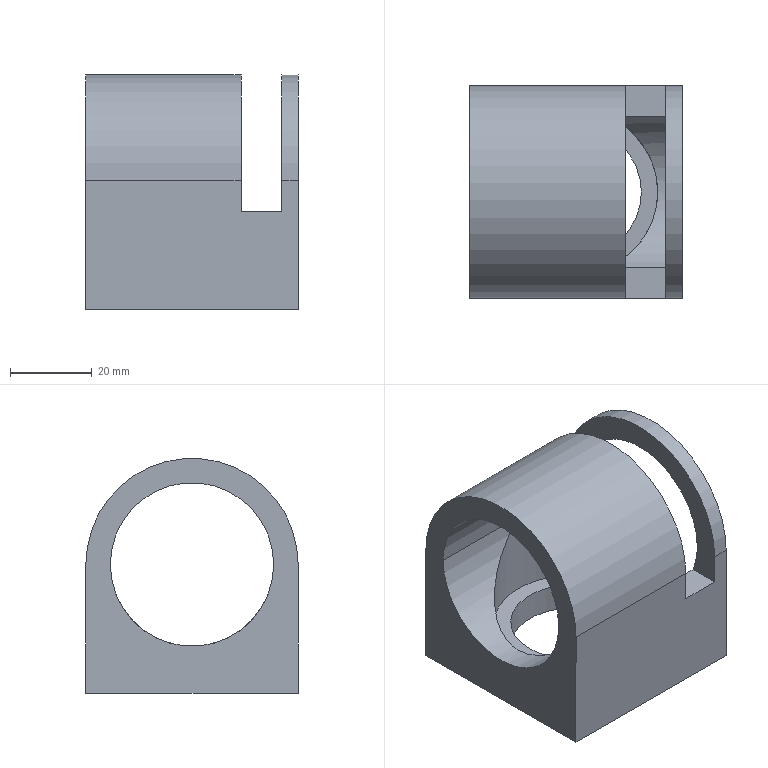Part | SolidWorks | features ICE 8, Extrusion 1 | 1 solid | 35 faces | box 52 x 52 x 57.532 mm | volume 52074 mm3 | cylinder 20 | plane 15 | commonest cylinder face diameters 4 x8 40 x6 32 x2 50 x2 52 x2
STEP:
#1=CARTESIAN_POINT('',(-20.,0.,10.));
#2=VERTEX_POINT('',#1);
#3=CARTESIAN_POINT('',(20.,0.,10.));
#4=VERTEX_POINT('',#3);
#5=CARTESIAN_POINT('',(0.,0.,10.));
#6=DIRECTION('',(0.,0.,1.));
#7=DIRECTION('',(1.,0.,0.));
#8=AXIS2_PLACEMENT_3D('',#5,#6,#7);
#9=CIRCLE('',#8,20.);
#10=EDGE_CURVE('',#2,#4,#9,.T.);
#11=ORIENTED_EDGE('',*,*,#10,.F.);
#12=CARTESIAN_POINT('',(-20.,0.,11.532));
#13=VERTEX_POINT('',#12);
#14=CARTESIAN_POINT('',(-20.,0.,10.));
#15=DIRECTION('',(0.,0.,1.));
#16=VECTOR('',#15,1000.);
#17=LINE('',#14,#16);
#18=EDGE_CURVE('',#2,#13,#17,.T.);
#19=ORIENTED_EDGE('',*,*,#18,.T.);
#20=CARTESIAN_POINT('',(0.,-20.,31.532));
#21=VERTEX_POINT('',#20);
#22=CARTESIAN_POINT('',(-20.,0.,11.532));
#23=CARTESIAN_POINT('',(-20.,-11.716,11.532));
#24=CARTESIAN_POINT('',(-11.716,-20.,19.816));
#25=CARTESIAN_POINT('',(0.,-20.,31.532));
#26=(BOUNDED_CURVE()B_SPLINE_CURVE(3,(#22,#23,#24,#25),.UNSPECIFIED.,.F.,.F.)B_SPLINE_CURVE_WITH_KNOTS((4,4),(3.142,4.712),.UNSPECIFIED.)CURVE()GEOMETRIC_REPRESENTATION_ITEM()RATIONAL_B_SPLINE_CURVE((1.,0.8047,0.8047,1.))REPRESENTATION_ITEM(''));
#27=EDGE_CURVE('',#13,#21,#26,.T.);
#28=ORIENTED_EDGE('',*,*,#27,.T.);
#29=CARTESIAN_POINT('',(20.,0.,11.532));
#30=VERTEX_POINT('',#29);
#31=CARTESIAN_POINT('',(0.,-20.,31.532));
#32=CARTESIAN_POINT('',(11.716,-20.,19.816));
#33=CARTESIAN_POINT('',(20.,-11.716,11.532));
#34=CARTESIAN_POINT('',(20.,0.,11.532));
#35=(BOUNDED_CURVE()B_SPLINE_CURVE(3,(#31,#32,#33,#34),.UNSPECIFIED.,.F.,.F.)B_SPLINE_CURVE_WITH_KNOTS((4,4),(1.571,3.142),.UNSPECIFIED.)CURVE()GEOMETRIC_REPRESENTATION_ITEM()RATIONAL_B_SPLINE_CURVE((1.,0.8047,0.8047,1.))REPRESENTATION_ITEM(''));
#36=EDGE_CURVE('',#21,#30,#35,.T.);
#37=ORIENTED_EDGE('',*,*,#36,.T.);
#38=CARTESIAN_POINT('',(20.,0.,10.));
#39=DIRECTION('',(0.,0.,1.));
#40=VECTOR('',#39,1000.);
#41=LINE('',#38,#40);
#42=EDGE_CURVE('',#4,#30,#41,.T.);
#43=ORIENTED_EDGE('',*,*,#42,.F.);
#44=EDGE_LOOP('',(#11,#19,#28,#37,#43));
#45=FACE_OUTER_BOUND('',#44,.T.);
#46=CARTESIAN_POINT('',(0.,0.,10.));
#47=DIRECTION('',(0.,0.,1.));
#48=DIRECTION('',(1.,0.,0.));
#49=AXIS2_PLACEMENT_3D('',#46,#47,#48);
#50=CYLINDRICAL_SURFACE('',#49,20.);
#51=ADVANCED_FACE('',(#45),#50,.F.);
#52=CARTESIAN_POINT('',(16.,0.,10.));
#53=VERTEX_POINT('',#52);
#54=CARTESIAN_POINT('',(-16.,0.,10.));
#55=VERTEX_POINT('',#54);
#56=CARTESIAN_POINT('',(0.,0.,10.));
#57=DIRECTION('',(0.,0.,-1.));
#58=DIRECTION('',(-1.,0.,0.));
#59=AXIS2_PLACEMENT_3D('',#56,#57,#58);
#60=CIRCLE('',#59,16.);
#61=EDGE_CURVE('',#53,#55,#60,.T.);
#62=ORIENTED_EDGE('',*,*,#61,.F.);
#63=CARTESIAN_POINT('',(16.,0.,3.));
#64=VERTEX_POINT('',#63);
#65=CARTESIAN_POINT('',(16.,0.,10.));
#66=DIRECTION('',(0.,0.,-1.));
#67=VECTOR('',#66,1000.);
#68=LINE('',#65,#67);
#69=EDGE_CURVE('',#53,#64,#68,.T.);
#70=ORIENTED_EDGE('',*,*,#69,.T.);
#71=CARTESIAN_POINT('',(-16.,0.,3.));
#72=VERTEX_POINT('',#71);
#73=CARTESIAN_POINT('',(0.,0.,3.));
#74=DIRECTION('',(0.,0.,-1.));
#75=DIRECTION('',(-1.,0.,0.));
#76=AXIS2_PLACEMENT_3D('',#73,#74,#75);
#77=CIRCLE('',#76,16.);
#78=EDGE_CURVE('',#64,#72,#77,.T.);
#79=ORIENTED_EDGE('',*,*,#78,.T.);
#80=CARTESIAN_POINT('',(-16.,0.,10.));
#81=DIRECTION('',(0.,0.,-1.));
#82=VECTOR('',#81,1000.);
#83=LINE('',#80,#82);
#84=EDGE_CURVE('',#55,#72,#83,.T.);
#85=ORIENTED_EDGE('',*,*,#84,.F.);
#86=EDGE_LOOP('',(#62,#70,#79,#85));
#87=FACE_OUTER_BOUND('',#86,.T.);
#88=CARTESIAN_POINT('',(0.,0.,10.));
#89=DIRECTION('',(0.,0.,-1.));
#90=DIRECTION('',(-1.,0.,0.));
#91=AXIS2_PLACEMENT_3D('',#88,#89,#90);
#92=CYLINDRICAL_SURFACE('',#91,16.);
#93=ADVANCED_FACE('',(#87),#92,.F.);
#94=CARTESIAN_POINT('',(25.,0.,3.));
#95=VERTEX_POINT('',#94);
#96=CARTESIAN_POINT('',(-25.,0.,3.));
#97=VERTEX_POINT('',#96);
#98=CARTESIAN_POINT('',(0.,0.,3.));
#99=DIRECTION('',(0.,0.,-1.));
#100=DIRECTION('',(-1.,0.,0.));
#101=AXIS2_PLACEMENT_3D('',#98,#99,#100);
#102=CIRCLE('',#101,25.);
#103=EDGE_CURVE('',#95,#97,#102,.T.);
#104=ORIENTED_EDGE('',*,*,#103,.F.);
#105=CARTESIAN_POINT('',(25.,0.,0.));
#106=VERTEX_POINT('',#105);
#107=CARTESIAN_POINT('',(25.,0.,3.));
#108=DIRECTION('',(0.,0.,-1.));
#109=VECTOR('',#108,1000.);
#110=LINE('',#107,#109);
#111=EDGE_CURVE('',#95,#106,#110,.T.);
#112=ORIENTED_EDGE('',*,*,#111,.T.);
#113=CARTESIAN_POINT('',(-25.,0.,0.));
#114=VERTEX_POINT('',#113);
#115=CARTESIAN_POINT('',(0.,0.,0.));
#116=DIRECTION('',(0.,0.,-1.));
#117=DIRECTION('',(-1.,0.,0.));
#118=AXIS2_PLACEMENT_3D('',#115,#116,#117);
#119=CIRCLE('',#118,25.);
#120=EDGE_CURVE('',#106,#114,#119,.T.);
#121=ORIENTED_EDGE('',*,*,#120,.T.);
#122=CARTESIAN_POINT('',(-25.,0.,3.));
#123=DIRECTION('',(0.,0.,-1.));
#124=VECTOR('',#123,1000.);
#125=LINE('',#122,#124);
#126=EDGE_CURVE('',#97,#114,#125,.T.);
#127=ORIENTED_EDGE('',*,*,#126,.F.);
#128=EDGE_LOOP('',(#104,#112,#121,#127));
#129=FACE_OUTER_BOUND('',#128,.T.);
#130=CARTESIAN_POINT('',(0.,0.,3.));
#131=DIRECTION('',(0.,0.,-1.));
#132=DIRECTION('',(-1.,0.,0.));
#133=AXIS2_PLACEMENT_3D('',#130,#131,#132);
#134=CYLINDRICAL_SURFACE('',#133,25.);
#135=ADVANCED_FACE('',(#129),#134,.F.);
#136=CARTESIAN_POINT('',(23.,-21.,10.));
#137=VERTEX_POINT('',#136);
#138=CARTESIAN_POINT('',(19.,-21.,10.));
#139=VERTEX_POINT('',#138);
#140=CARTESIAN_POINT('',(21.,-21.,10.));
#141=DIRECTION('',(0.,0.,-1.));
#142=DIRECTION('',(1.,0.,0.));
#143=AXIS2_PLACEMENT_3D('',#140,#141,#142);
#144=CIRCLE('',#143,2.);
#145=EDGE_CURVE('',#137,#139,#144,.T.);
#146=ORIENTED_EDGE('',*,*,#145,.F.);
#147=CARTESIAN_POINT('',(23.,-21.,0.));
#148=VERTEX_POINT('',#147);
#149=CARTESIAN_POINT('',(23.,-21.,10.));
#150=DIRECTION('',(0.,0.,-1.));
#151=VECTOR('',#150,1000.);
#152=LINE('',#149,#151);
#153=EDGE_CURVE('',#137,#148,#152,.T.);
#154=ORIENTED_EDGE('',*,*,#153,.T.);
#155=CARTESIAN_POINT('',(19.,-21.,0.));
#156=VERTEX_POINT('',#155);
#157=CARTESIAN_POINT('',(21.,-21.,0.));
#158=DIRECTION('',(0.,0.,-1.));
#159=DIRECTION('',(1.,0.,0.));
#160=AXIS2_PLACEMENT_3D('',#157,#158,#159);
#161=CIRCLE('',#160,2.);
#162=EDGE_CURVE('',#148,#156,#161,.T.);
#163=ORIENTED_EDGE('',*,*,#162,.T.);
#164=CARTESIAN_POINT('',(19.,-21.,10.));
#165=DIRECTION('',(0.,0.,-1.));
#166=VECTOR('',#165,1000.);
#167=LINE('',#164,#166);
#168=EDGE_CURVE('',#139,#156,#167,.T.);
#169=ORIENTED_EDGE('',*,*,#168,.F.);
#170=EDGE_LOOP('',(#146,#154,#163,#169));
#171=FACE_OUTER_BOUND('',#170,.T.);
#172=CARTESIAN_POINT('',(21.,-21.,10.));
#173=DIRECTION('',(0.,0.,-1.));
#174=DIRECTION('',(-1.,0.,0.));
#175=AXIS2_PLACEMENT_3D('',#172,#173,#174);
#176=CYLINDRICAL_SURFACE('',#175,2.);
#177=ADVANCED_FACE('',(#171),#176,.F.);
#178=CARTESIAN_POINT('',(-19.,-21.,10.));
#179=VERTEX_POINT('',#178);
#180=CARTESIAN_POINT('',(-23.,-21.,10.));
#181=VERTEX_POINT('',#180);
#182=CARTESIAN_POINT('',(-21.,-21.,10.));
#183=DIRECTION('',(0.,0.,-1.));
#184=DIRECTION('',(-1.,0.,0.));
#185=AXIS2_PLACEMENT_3D('',#182,#183,#184);
#186=CIRCLE('',#185,2.);
#187=EDGE_CURVE('',#179,#181,#186,.T.);
#188=ORIENTED_EDGE('',*,*,#187,.F.);
#189=CARTESIAN_POINT('',(-19.,-21.,0.));
#190=VERTEX_POINT('',#189);
#191=CARTESIAN_POINT('',(-19.,-21.,10.));
#192=DIRECTION('',(0.,0.,-1.));
#193=VECTOR('',#192,1000.);
#194=LINE('',#191,#193);
#195=EDGE_CURVE('',#179,#190,#194,.T.);
#196=ORIENTED_EDGE('',*,*,#195,.T.);
#197=CARTESIAN_POINT('',(-23.,-21.,0.));
#198=VERTEX_POINT('',#197);
#199=CARTESIAN_POINT('',(-21.,-21.,0.));
#200=DIRECTION('',(0.,0.,-1.));
#201=DIRECTION('',(-1.,0.,0.));
#202=AXIS2_PLACEMENT_3D('',#199,#200,#201);
#203=CIRCLE('',#202,2.);
#204=EDGE_CURVE('',#190,#198,#203,.T.);
#205=ORIENTED_EDGE('',*,*,#204,.T.);
#206=CARTESIAN_POINT('',(-23.,-21.,10.));
#207=DIRECTION('',(0.,0.,-1.));
#208=VECTOR('',#207,1000.);
#209=LINE('',#206,#208);
#210=EDGE_CURVE('',#181,#198,#209,.T.);
#211=ORIENTED_EDGE('',*,*,#210,.F.);
#212=EDGE_LOOP('',(#188,#196,#205,#211));
#213=FACE_OUTER_BOUND('',#212,.T.);
#214=CARTESIAN_POINT('',(-21.,-21.,10.));
#215=DIRECTION('',(0.,0.,-1.));
#216=DIRECTION('',(-1.,0.,0.));
#217=AXIS2_PLACEMENT_3D('',#214,#215,#216);
#218=CYLINDRICAL_SURFACE('',#217,2.);
#219=ADVANCED_FACE('',(#213),#218,.F.);
#220=CARTESIAN_POINT('',(-19.,21.,10.));
#221=VERTEX_POINT('',#220);
#222=CARTESIAN_POINT('',(-23.,21.,10.));
#223=VERTEX_POINT('',#222);
#224=CARTESIAN_POINT('',(-21.,21.,10.));
#225=DIRECTION('',(0.,0.,-1.));
#226=DIRECTION('',(1.,0.,0.));
#227=AXIS2_PLACEMENT_3D('',#224,#225,#226);
#228=CIRCLE('',#227,2.);
#229=EDGE_CURVE('',#221,#223,#228,.T.);
#230=ORIENTED_EDGE('',*,*,#229,.F.);
#231=CARTESIAN_POINT('',(-19.,21.,0.));
#232=VERTEX_POINT('',#231);
#233=CARTESIAN_POINT('',(-19.,21.,10.));
#234=DIRECTION('',(0.,0.,-1.));
#235=VECTOR('',#234,1000.);
#236=LINE('',#233,#235);
#237=EDGE_CURVE('',#221,#232,#236,.T.);
#238=ORIENTED_EDGE('',*,*,#237,.T.);
#239=CARTESIAN_POINT('',(-23.,21.,0.));
#240=VERTEX_POINT('',#239);
#241=CARTESIAN_POINT('',(-21.,21.,0.));
#242=DIRECTION('',(0.,0.,-1.));
#243=DIRECTION('',(1.,0.,0.));
#244=AXIS2_PLACEMENT_3D('',#241,#242,#243);
#245=CIRCLE('',#244,2.);
#246=EDGE_CURVE('',#232,#240,#245,.T.);
#247=ORIENTED_EDGE('',*,*,#246,.T.);
#248=CARTESIAN_POINT('',(-23.,21.,10.));
#249=DIRECTION('',(0.,0.,-1.));
#250=VECTOR('',#249,1000.);
#251=LINE('',#248,#250);
#252=EDGE_CURVE('',#223,#240,#251,.T.);
#253=ORIENTED_EDGE('',*,*,#252,.F.);
#254=EDGE_LOOP('',(#230,#238,#247,#253));
#255=FACE_OUTER_BOUND('',#254,.T.);
#256=CARTESIAN_POINT('',(-21.,21.,10.));
#257=DIRECTION('',(0.,0.,-1.));
#258=DIRECTION('',(-1.,0.,0.));
#259=AXIS2_PLACEMENT_3D('',#256,#257,#258);
#260=CYLINDRICAL_SURFACE('',#259,2.);
#261=ADVANCED_FACE('',(#255),#260,.F.);
#262=CARTESIAN_POINT('',(23.,21.,10.));
#263=VERTEX_POINT('',#262);
#264=CARTESIAN_POINT('',(19.,21.,10.));
#265=VERTEX_POINT('',#264);
#266=CARTESIAN_POINT('',(21.,21.,10.));
#267=DIRECTION('',(0.,0.,-1.));
#268=DIRECTION('',(-1.,0.,0.));
#269=AXIS2_PLACEMENT_3D('',#266,#267,#268);
#270=CIRCLE('',#269,2.);
#271=EDGE_CURVE('',#263,#265,#270,.T.);
#272=ORIENTED_EDGE('',*,*,#271,.F.);
#273=CARTESIAN_POINT('',(23.,21.,0.));
#274=VERTEX_POINT('',#273);
#275=CARTESIAN_POINT('',(23.,21.,10.));
#276=DIRECTION('',(0.,0.,-1.));
#277=VECTOR('',#276,1000.);
#278=LINE('',#275,#277);
#279=EDGE_CURVE('',#263,#274,#278,.T.);
#280=ORIENTED_EDGE('',*,*,#279,.T.);
#281=CARTESIAN_POINT('',(19.,21.,0.));
#282=VERTEX_POINT('',#281);
#283=CARTESIAN_POINT('',(21.,21.,0.));
#284=DIRECTION('',(0.,0.,-1.));
#285=DIRECTION('',(-1.,0.,0.));
#286=AXIS2_PLACEMENT_3D('',#283,#284,#285);
#287=CIRCLE('',#286,2.);
#288=EDGE_CURVE('',#274,#282,#287,.T.);
#289=ORIENTED_EDGE('',*,*,#288,.T.);
#290=CARTESIAN_POINT('',(19.,21.,10.));
#291=DIRECTION('',(0.,0.,-1.));
#292=VECTOR('',#291,1000.);
#293=LINE('',#290,#292);
#294=EDGE_CURVE('',#265,#282,#293,.T.);
#295=ORIENTED_EDGE('',*,*,#294,.F.);
#296=EDGE_LOOP('',(#272,#280,#289,#295));
#297=FACE_OUTER_BOUND('',#296,.T.);
#298=CARTESIAN_POINT('',(21.,21.,10.));
#299=DIRECTION('',(0.,0.,-1.));
#300=DIRECTION('',(-1.,0.,0.));
#301=AXIS2_PLACEMENT_3D('',#298,#299,#300);
#302=CYLINDRICAL_SURFACE('',#301,2.);
#303=ADVANCED_FACE('',(#297),#302,.F.);
#304=CARTESIAN_POINT('',(26.,20.,31.532));
#305=VERTEX_POINT('',#304);
#306=CARTESIAN_POINT('',(26.,-20.,31.532));
#307=VERTEX_POINT('',#306);
#308=CARTESIAN_POINT('',(26.,0.,31.532));
#309=DIRECTION('',(-1.,0.,0.));
#310=DIRECTION('',(0.,-1.,0.));
#311=AXIS2_PLACEMENT_3D('',#308,#309,#310);
#312=CIRCLE('',#311,20.);
#313=EDGE_CURVE('',#305,#307,#312,.T.);
#314=ORIENTED_EDGE('',*,*,#313,.F.);
#315=CARTESIAN_POINT('',(22.,20.,31.532));
#316=VERTEX_POINT('',#315);
#317=CARTESIAN_POINT('',(26.,20.,31.532));
#318=DIRECTION('',(-1.,0.,0.));
#319=VECTOR('',#318,1000.);
#320=LINE('',#317,#319);
#321=EDGE_CURVE('',#305,#316,#320,.T.);
#322=ORIENTED_EDGE('',*,*,#321,.T.);
#323=CARTESIAN_POINT('',(22.,18.528,24.));
#324=VERTEX_POINT('',#323);
#325=CARTESIAN_POINT('',(22.,0.,31.532));
#326=DIRECTION('',(-1.,0.,0.));
#327=DIRECTION('',(0.,1.,0.));
#328=AXIS2_PLACEMENT_3D('',#325,#326,#327);
#329=CIRCLE('',#328,20.);
#330=EDGE_CURVE('',#316,#324,#329,.T.);
#331=ORIENTED_EDGE('',*,*,#330,.T.);
#332=CARTESIAN_POINT('',(12.,18.528,24.));
#333=VERTEX_POINT('',#332);
#334=CARTESIAN_POINT('',(26.,18.528,24.));
#335=DIRECTION('',(-1.,0.,0.));
#336=VECTOR('',#335,1000.);
#337=LINE('',#334,#336);
#338=EDGE_CURVE('',#324,#333,#337,.T.);
#339=ORIENTED_EDGE('',*,*,#338,.T.);
#340=CARTESIAN_POINT('',(12.,20.,31.532));
#341=VERTEX_POINT('',#340);
#342=CARTESIAN_POINT('',(12.,0.,31.532));
#343=DIRECTION('',(-1.,0.,0.));
#344=DIRECTION('',(0.,1.,0.));
#345=AXIS2_PLACEMENT_3D('',#342,#343,#344);
#346=CIRCLE('',#345,20.);
#347=EDGE_CURVE('',#341,#333,#346,.T.);
#348=ORIENTED_EDGE('',*,*,#347,.F.);
#349=CARTESIAN_POINT('',(0.,20.,31.532));
#350=VERTEX_POINT('',#349);
#351=CARTESIAN_POINT('',(26.,20.,31.532));
#352=DIRECTION('',(-1.,0.,0.));
#353=VECTOR('',#352,1000.);
#354=LINE('',#351,#353);
#355=EDGE_CURVE('',#341,#350,#354,.T.);
#356=ORIENTED_EDGE('',*,*,#355,.T.);
#357=CARTESIAN_POINT('',(20.,0.,11.532));
#358=CARTESIAN_POINT('',(20.,11.716,11.532));
#359=CARTESIAN_POINT('',(11.716,20.,19.816));
#360=CARTESIAN_POINT('',(0.,20.,31.532));
#361=(BOUNDED_CURVE()B_SPLINE_CURVE(3,(#357,#358,#359,#360),.UNSPECIFIED.,.F.,.F.)B_SPLINE_CURVE_WITH_KNOTS((4,4),(3.142,4.712),.UNSPECIFIED.)CURVE()GEOMETRIC_REPRESENTATION_ITEM()RATIONAL_B_SPLINE_CURVE((1.,0.8047,0.8047,1.))REPRESENTATION_ITEM(''));
#362=EDGE_CURVE('',#30,#350,#361,.T.);
#363=ORIENTED_EDGE('',*,*,#362,.F.);
#364=ORIENTED_EDGE('',*,*,#36,.F.);
#365=CARTESIAN_POINT('',(12.,-20.,31.532));
#366=VERTEX_POINT('',#365);
#367=CARTESIAN_POINT('',(26.,-20.,31.532));
#368=DIRECTION('',(-1.,0.,0.));
#369=VECTOR('',#368,1000.);
#370=LINE('',#367,#369);
#371=EDGE_CURVE('',#366,#21,#370,.T.);
#372=ORIENTED_EDGE('',*,*,#371,.F.);
#373=CARTESIAN_POINT('',(12.,-18.528,24.));
#374=VERTEX_POINT('',#373);
#375=CARTESIAN_POINT('',(12.,0.,31.532));
#376=DIRECTION('',(-1.,0.,0.));
#377=DIRECTION('',(0.,1.,0.));
#378=AXIS2_PLACEMENT_3D('',#375,#376,#377);
#379=CIRCLE('',#378,20.);
#380=EDGE_CURVE('',#374,#366,#379,.T.);
#381=ORIENTED_EDGE('',*,*,#380,.F.);
#382=CARTESIAN_POINT('',(22.,-18.528,24.));
#383=VERTEX_POINT('',#382);
#384=CARTESIAN_POINT('',(26.,-18.528,24.));
#385=DIRECTION('',(1.,0.,0.));
#386=VECTOR('',#385,1000.);
#387=LINE('',#384,#386);
#388=EDGE_CURVE('',#374,#383,#387,.T.);
#389=ORIENTED_EDGE('',*,*,#388,.T.);
#390=CARTESIAN_POINT('',(22.,-20.,31.532));
#391=VERTEX_POINT('',#390);
#392=CARTESIAN_POINT('',(22.,0.,31.532));
#393=DIRECTION('',(-1.,0.,0.));
#394=DIRECTION('',(0.,1.,0.));
#395=AXIS2_PLACEMENT_3D('',#392,#393,#394);
#396=CIRCLE('',#395,20.);
#397=EDGE_CURVE('',#383,#391,#396,.T.);
#398=ORIENTED_EDGE('',*,*,#397,.T.);
#399=CARTESIAN_POINT('',(26.,-20.,31.532));
#400=DIRECTION('',(-1.,0.,0.));
#401=VECTOR('',#400,1000.);
#402=LINE('',#399,#401);
#403=EDGE_CURVE('',#307,#391,#402,.T.);
#404=ORIENTED_EDGE('',*,*,#403,.F.);
#405=EDGE_LOOP('',(#314,#322,#331,#339,#348,#356,#363,#364,#372,#381,#389,#398,#404));
#406=FACE_OUTER_BOUND('',#405,.T.);
#407=CARTESIAN_POINT('',(26.,0.,31.532));
#408=DIRECTION('',(-1.,0.,0.));
#409=DIRECTION('',(0.,-1.,0.));
#410=AXIS2_PLACEMENT_3D('',#407,#408,#409);
#411=CYLINDRICAL_SURFACE('',#410,20.);
#412=ADVANCED_FACE('',(#406),#411,.F.);
#413=ORIENTED_EDGE('',*,*,#321,.F.);
#414=CARTESIAN_POINT('',(26.,0.,31.532));
#415=DIRECTION('',(-1.,0.,0.));
#416=DIRECTION('',(0.,-1.,0.));
#417=AXIS2_PLACEMENT_3D('',#414,#415,#416);
#418=CIRCLE('',#417,20.);
#419=EDGE_CURVE('',#307,#305,#418,.T.);
#420=ORIENTED_EDGE('',*,*,#419,.F.);
#421=ORIENTED_EDGE('',*,*,#403,.T.);
#422=CARTESIAN_POINT('',(22.,0.,31.532));
#423=DIRECTION('',(-1.,0.,0.));
#424=DIRECTION('',(0.,1.,0.));
#425=AXIS2_PLACEMENT_3D('',#422,#423,#424);
#426=CIRCLE('',#425,20.);
#427=EDGE_CURVE('',#391,#316,#426,.T.);
#428=ORIENTED_EDGE('',*,*,#427,.T.);
#429=EDGE_LOOP('',(#413,#420,#421,#428));
#430=FACE_OUTER_BOUND('',#429,.T.);
#431=CARTESIAN_POINT('',(26.,0.,31.532));
#432=DIRECTION('',(-1.,0.,0.));
#433=DIRECTION('',(0.,-1.,0.));
#434=AXIS2_PLACEMENT_3D('',#431,#432,#433);
#435=CYLINDRICAL_SURFACE('',#434,20.);
#436=ADVANCED_FACE('',(#430),#435,.F.);
#437=CARTESIAN_POINT('',(0.,20.,31.532));
#438=CARTESIAN_POINT('',(-11.716,20.,19.816));
#439=CARTESIAN_POINT('',(-20.,11.716,11.532));
#440=CARTESIAN_POINT('',(-20.,0.,11.532));
#441=(BOUNDED_CURVE()B_SPLINE_CURVE(3,(#437,#438,#439,#440),.UNSPECIFIED.,.F.,.F.)B_SPLINE_CURVE_WITH_KNOTS((4,4),(1.571,3.142),.UNSPECIFIED.)CURVE()GEOMETRIC_REPRESENTATION_ITEM()RATIONAL_B_SPLINE_CURVE((1.,0.8047,0.8047,1.))REPRESENTATION_ITEM(''));
#442=EDGE_CURVE('',#350,#13,#441,.T.);
#443=ORIENTED_EDGE('',*,*,#442,.F.);
#444=CARTESIAN_POINT('',(-26.,20.,31.532));
#445=VERTEX_POINT('',#444);
#446=CARTESIAN_POINT('',(26.,20.,31.532));
#447=DIRECTION('',(-1.,0.,0.));
#448=VECTOR('',#447,1000.);
#449=LINE('',#446,#448);
#450=EDGE_CURVE('',#350,#445,#449,.T.);
#451=ORIENTED_EDGE('',*,*,#450,.T.);
#452=CARTESIAN_POINT('',(-26.,-20.,31.532));
#453=VERTEX_POINT('',#452);
#454=CARTESIAN_POINT('',(-26.,0.,31.532));
#455=DIRECTION('',(-1.,0.,0.));
#456=DIRECTION('',(0.,-1.,0.));
#457=AXIS2_PLACEMENT_3D('',#454,#455,#456);
#458=CIRCLE('',#457,20.);
#459=EDGE_CURVE('',#445,#453,#458,.T.);
#460=ORIENTED_EDGE('',*,*,#459,.T.);
#461=CARTESIAN_POINT('',(26.,-20.,31.532));
#462=DIRECTION('',(-1.,0.,0.));
#463=VECTOR('',#462,1000.);
#464=LINE('',#461,#463);
#465=EDGE_CURVE('',#21,#453,#464,.T.);
#466=ORIENTED_EDGE('',*,*,#465,.F.);
#467=ORIENTED_EDGE('',*,*,#27,.F.);
#468=EDGE_LOOP('',(#443,#451,#460,#466,#467));
#469=FACE_OUTER_BOUND('',#468,.T.);
#470=CARTESIAN_POINT('',(26.,0.,31.532));
#471=DIRECTION('',(-1.,0.,0.));
#472=DIRECTION('',(0.,-1.,0.));
#473=AXIS2_PLACEMENT_3D('',#470,#471,#472);
#474=CYLINDRICAL_SURFACE('',#473,20.);
#475=ADVANCED_FACE('',(#469),#474,.F.);
#476=CARTESIAN_POINT('',(12.,-26.,31.532));
#477=VERTEX_POINT('',#476);
#478=CARTESIAN_POINT('',(12.,-26.,24.));
#479=VERTEX_POINT('',#478);
#480=CARTESIAN_POINT('',(12.,-26.,10.));
#481=DIRECTION('',(0.,0.,-1.));
#482=VECTOR('',#481,1000.);
#483=LINE('',#480,#482);
#484=EDGE_CURVE('',#477,#479,#483,.T.);
#485=ORIENTED_EDGE('',*,*,#484,.F.);
#486=CARTESIAN_POINT('',(-26.,-26.,31.532));
#487=VERTEX_POINT('',#486);
#488=CARTESIAN_POINT('',(26.,-26.,31.532));
#489=DIRECTION('',(-1.,0.,0.));
#490=VECTOR('',#489,1000.);
#491=LINE('',#488,#490);
#492=EDGE_CURVE('',#477,#487,#491,.T.);
#493=ORIENTED_EDGE('',*,*,#492,.T.);
#494=CARTESIAN_POINT('',(-26.,-26.,0.));
#495=VERTEX_POINT('',#494);
#496=CARTESIAN_POINT('',(-26.,-26.,10.));
#497=DIRECTION('',(0.,0.,-1.));
#498=VECTOR('',#497,1000.);
#499=LINE('',#496,#498);
#500=EDGE_CURVE('',#487,#495,#499,.T.);
#501=ORIENTED_EDGE('',*,*,#500,.T.);
#502=CARTESIAN_POINT('',(26.,-26.,0.));
#503=VERTEX_POINT('',#502);
#504=CARTESIAN_POINT('',(-26.,-26.,0.));
#505=DIRECTION('',(1.,0.,0.));
#506=VECTOR('',#505,1000.);
#507=LINE('',#504,#506);
#508=EDGE_CURVE('',#495,#503,#507,.T.);
#509=ORIENTED_EDGE('',*,*,#508,.T.);
#510=CARTESIAN_POINT('',(26.,-26.,31.532));
#511=VERTEX_POINT('',#510);
#512=CARTESIAN_POINT('',(26.,-26.,10.));
#513=DIRECTION('',(0.,0.,-1.));
#514=VECTOR('',#513,1000.);
#515=LINE('',#512,#514);
#516=EDGE_CURVE('',#511,#503,#515,.T.);
#517=ORIENTED_EDGE('',*,*,#516,.F.);
#518=CARTESIAN_POINT('',(22.,-26.,31.532));
#519=VERTEX_POINT('',#518);
#520=CARTESIAN_POINT('',(26.,-26.,31.532));
#521=DIRECTION('',(-1.,0.,0.));
#522=VECTOR('',#521,1000.);
#523=LINE('',#520,#522);
#524=EDGE_CURVE('',#511,#519,#523,.T.);
#525=ORIENTED_EDGE('',*,*,#524,.T.);
#526=CARTESIAN_POINT('',(22.,-26.,24.));
#527=VERTEX_POINT('',#526);
#528=CARTESIAN_POINT('',(22.,-26.,10.));
#529=DIRECTION('',(0.,0.,-1.));
#530=VECTOR('',#529,1000.);
#531=LINE('',#528,#530);
#532=EDGE_CURVE('',#519,#527,#531,.T.);
#533=ORIENTED_EDGE('',*,*,#532,.T.);
#534=CARTESIAN_POINT('',(-26.,-26.,24.));
#535=DIRECTION('',(-1.,0.,0.));
#536=VECTOR('',#535,1000.);
#537=LINE('',#534,#536);
#538=EDGE_CURVE('',#527,#479,#537,.T.);
#539=ORIENTED_EDGE('',*,*,#538,.T.);
#540=EDGE_LOOP('',(#485,#493,#501,#509,#517,#525,#533,#539));
#541=FACE_OUTER_BOUND('',#540,.T.);
#542=CARTESIAN_POINT('',(-26.,-26.,10.));
#543=DIRECTION('',(0.,1.,0.));
#544=DIRECTION('',(0.,0.,1.));
#545=AXIS2_PLACEMENT_3D('',#542,#543,#544);
#546=PLANE('',#545);
#547=ADVANCED_FACE('',(#541),#546,.F.);
#548=CARTESIAN_POINT('',(12.,26.,24.));
#549=VERTEX_POINT('',#548);
#550=CARTESIAN_POINT('',(12.,26.,31.532));
#551=VERTEX_POINT('',#550);
#552=CARTESIAN_POINT('',(12.,26.,10.));
#553=DIRECTION('',(0.,0.,1.));
#554=VECTOR('',#553,1000.);
#555=LINE('',#552,#554);
#556=EDGE_CURVE('',#549,#551,#555,.T.);
#557=ORIENTED_EDGE('',*,*,#556,.F.);
#558=CARTESIAN_POINT('',(22.,26.,24.));
#559=VERTEX_POINT('',#558);
#560=CARTESIAN_POINT('',(26.,26.,24.));
#561=DIRECTION('',(1.,0.,0.));
#562=VECTOR('',#561,1000.);
#563=LINE('',#560,#562);
#564=EDGE_CURVE('',#549,#559,#563,.T.);
#565=ORIENTED_EDGE('',*,*,#564,.T.);
#566=CARTESIAN_POINT('',(22.,26.,31.532));
#567=VERTEX_POINT('',#566);
#568=CARTESIAN_POINT('',(22.,26.,10.));
#569=DIRECTION('',(0.,0.,1.));
#570=VECTOR('',#569,1000.);
#571=LINE('',#568,#570);
#572=EDGE_CURVE('',#559,#567,#571,.T.);
#573=ORIENTED_EDGE('',*,*,#572,.T.);
#574=CARTESIAN_POINT('',(26.,26.,31.532));
#575=VERTEX_POINT('',#574);
#576=CARTESIAN_POINT('',(26.,26.,31.532));
#577=DIRECTION('',(-1.,0.,0.));
#578=VECTOR('',#577,1000.);
#579=LINE('',#576,#578);
#580=EDGE_CURVE('',#575,#567,#579,.T.);
#581=ORIENTED_EDGE('',*,*,#580,.F.);
#582=CARTESIAN_POINT('',(26.,26.,0.));
#583=VERTEX_POINT('',#582);
#584=CARTESIAN_POINT('',(26.,26.,10.));
#585=DIRECTION('',(0.,0.,-1.));
#586=VECTOR('',#585,1000.);
#587=LINE('',#584,#586);
#588=EDGE_CURVE('',#575,#583,#587,.T.);
#589=ORIENTED_EDGE('',*,*,#588,.T.);
#590=CARTESIAN_POINT('',(-26.,26.,0.));
#591=VERTEX_POINT('',#590);
#592=CARTESIAN_POINT('',(26.,26.,0.));
#593=DIRECTION('',(-1.,0.,0.));
#594=VECTOR('',#593,1000.);
#595=LINE('',#592,#594);
#596=EDGE_CURVE('',#583,#591,#595,.T.);
#597=ORIENTED_EDGE('',*,*,#596,.T.);
#598=CARTESIAN_POINT('',(-26.,26.,31.532));
#599=VERTEX_POINT('',#598);
#600=CARTESIAN_POINT('',(-26.,26.,10.));
#601=DIRECTION('',(0.,0.,-1.));
#602=VECTOR('',#601,1000.);
#603=LINE('',#600,#602);
#604=EDGE_CURVE('',#599,#591,#603,.T.);
#605=ORIENTED_EDGE('',*,*,#604,.F.);
#606=CARTESIAN_POINT('',(26.,26.,31.532));
#607=DIRECTION('',(-1.,0.,0.));
#608=VECTOR('',#607,1000.);
#609=LINE('',#606,#608);
#610=EDGE_CURVE('',#551,#599,#609,.T.);
#611=ORIENTED_EDGE('',*,*,#610,.F.);
#612=EDGE_LOOP('',(#557,#565,#573,#581,#589,#597,#605,#611));
#613=FACE_OUTER_BOUND('',#612,.T.);
#614=CARTESIAN_POINT('',(26.,26.,10.));
#615=DIRECTION('',(0.,-1.,0.));
#616=DIRECTION('',(0.,0.,-1.));
#617=AXIS2_PLACEMENT_3D('',#614,#615,#616);
#618=PLANE('',#617);
#619=ADVANCED_FACE('',(#613),#618,.F.);
#620=ORIENTED_EDGE('',*,*,#492,.F.);
#621=CARTESIAN_POINT('',(12.,0.,31.532));
#622=DIRECTION('',(-1.,0.,0.));
#623=DIRECTION('',(0.,1.,0.));
#624=AXIS2_PLACEMENT_3D('',#621,#622,#623);
#625=CIRCLE('',#624,26.);
#626=EDGE_CURVE('',#477,#551,#625,.T.);
#627=ORIENTED_EDGE('',*,*,#626,.T.);
#628=ORIENTED_EDGE('',*,*,#610,.T.);
#629=CARTESIAN_POINT('',(-26.,0.,31.532));
#630=DIRECTION('',(-1.,0.,0.));
#631=DIRECTION('',(0.,-1.,0.));
#632=AXIS2_PLACEMENT_3D('',#629,#630,#631);
#633=CIRCLE('',#632,26.);
#634=EDGE_CURVE('',#487,#599,#633,.T.);
#635=ORIENTED_EDGE('',*,*,#634,.F.);
#636=EDGE_LOOP('',(#620,#627,#628,#635));
#637=FACE_OUTER_BOUND('',#636,.T.);
#638=CARTESIAN_POINT('',(26.,0.,31.532));
#639=DIRECTION('',(-1.,0.,0.));
#640=DIRECTION('',(0.,-1.,0.));
#641=AXIS2_PLACEMENT_3D('',#638,#639,#640);
#642=CYLINDRICAL_SURFACE('',#641,26.);
#643=ADVANCED_FACE('',(#637),#642,.T.);
#644=ORIENTED_EDGE('',*,*,#355,.F.);
#645=CARTESIAN_POINT('',(12.,0.,31.532));
#646=DIRECTION('',(-1.,0.,0.));
#647=DIRECTION('',(0.,1.,0.));
#648=AXIS2_PLACEMENT_3D('',#645,#646,#647);
#649=CIRCLE('',#648,20.);
#650=EDGE_CURVE('',#366,#341,#649,.T.);
#651=ORIENTED_EDGE('',*,*,#650,.F.);
#652=ORIENTED_EDGE('',*,*,#371,.T.);
#653=ORIENTED_EDGE('',*,*,#465,.T.);
#654=CARTESIAN_POINT('',(-26.,0.,31.532));
#655=DIRECTION('',(-1.,0.,0.));
#656=DIRECTION('',(0.,-1.,0.));
#657=AXIS2_PLACEMENT_3D('',#654,#655,#656);
#658=CIRCLE('',#657,20.);
#659=EDGE_CURVE('',#453,#445,#658,.T.);
#660=ORIENTED_EDGE('',*,*,#659,.T.);
#661=ORIENTED_EDGE('',*,*,#450,.F.);
#662=EDGE_LOOP('',(#644,#651,#652,#653,#660,#661));
#663=FACE_OUTER_BOUND('',#662,.T.);
#664=CARTESIAN_POINT('',(26.,0.,31.532));
#665=DIRECTION('',(-1.,0.,0.));
#666=DIRECTION('',(0.,-1.,0.));
#667=AXIS2_PLACEMENT_3D('',#664,#665,#666);
#668=CYLINDRICAL_SURFACE('',#667,20.);
#669=ADVANCED_FACE('',(#663),#668,.F.);
#670=ORIENTED_EDGE('',*,*,#419,.T.);
#671=ORIENTED_EDGE('',*,*,#313,.T.);
#672=EDGE_LOOP('',(#670,#671));
#673=FACE_BOUND('',#672,.T.);
#674=CARTESIAN_POINT('',(26.,-26.,0.));
#675=DIRECTION('',(0.,1.,0.));
#676=VECTOR('',#675,1000.);
#677=LINE('',#674,#676);
#678=EDGE_CURVE('',#503,#583,#677,.T.);
#679=ORIENTED_EDGE('',*,*,#678,.T.);
#680=ORIENTED_EDGE('',*,*,#588,.F.);
#681=CARTESIAN_POINT('',(26.,0.,31.532));
#682=DIRECTION('',(-1.,0.,0.));
#683=DIRECTION('',(0.,-1.,0.));
#684=AXIS2_PLACEMENT_3D('',#681,#682,#683);
#685=CIRCLE('',#684,26.);
#686=EDGE_CURVE('',#511,#575,#685,.T.);
#687=ORIENTED_EDGE('',*,*,#686,.F.);
#688=ORIENTED_EDGE('',*,*,#516,.T.);
#689=EDGE_LOOP('',(#679,#680,#687,#688));
#690=FACE_OUTER_BOUND('',#689,.T.);
#691=CARTESIAN_POINT('',(26.,-26.,10.));
#692=DIRECTION('',(-1.,0.,0.));
#693=DIRECTION('',(0.,-1.,0.));
#694=AXIS2_PLACEMENT_3D('',#691,#692,#693);
#695=PLANE('',#694);
#696=ADVANCED_FACE('',(#673,#690),#695,.F.);
#697=ORIENTED_EDGE('',*,*,#659,.F.);
#698=ORIENTED_EDGE('',*,*,#459,.F.);
#699=EDGE_LOOP('',(#697,#698));
#700=FACE_BOUND('',#699,.T.);
#701=CARTESIAN_POINT('',(-26.,26.,0.));
#702=DIRECTION('',(0.,-1.,0.));
#703=VECTOR('',#702,1000.);
#704=LINE('',#701,#703);
#705=EDGE_CURVE('',#591,#495,#704,.T.);
#706=ORIENTED_EDGE('',*,*,#705,.T.);
#707=ORIENTED_EDGE('',*,*,#500,.F.);
#708=ORIENTED_EDGE('',*,*,#634,.T.);
#709=ORIENTED_EDGE('',*,*,#604,.T.);
#710=EDGE_LOOP('',(#706,#707,#708,#709));
#711=FACE_OUTER_BOUND('',#710,.T.);
#712=CARTESIAN_POINT('',(-26.,26.,10.));
#713=DIRECTION('',(1.,0.,0.));
#714=DIRECTION('',(0.,1.,0.));
#715=AXIS2_PLACEMENT_3D('',#712,#713,#714);
#716=PLANE('',#715);
#717=ADVANCED_FACE('',(#700,#711),#716,.F.);
#718=CARTESIAN_POINT('',(0.,0.,0.));
#719=DIRECTION('',(0.,0.,-1.));
#720=DIRECTION('',(-1.,0.,0.));
#721=AXIS2_PLACEMENT_3D('',#718,#719,#720);
#722=CIRCLE('',#721,25.);
#723=EDGE_CURVE('',#114,#106,#722,.T.);
#724=ORIENTED_EDGE('',*,*,#723,.F.);
#725=ORIENTED_EDGE('',*,*,#120,.F.);
#726=EDGE_LOOP('',(#724,#725));
#727=FACE_BOUND('',#726,.T.);
#728=CARTESIAN_POINT('',(21.,-21.,0.));
#729=DIRECTION('',(0.,0.,-1.));
#730=DIRECTION('',(1.,0.,0.));
#731=AXIS2_PLACEMENT_3D('',#728,#729,#730);
#732=CIRCLE('',#731,2.);
#733=EDGE_CURVE('',#156,#148,#732,.T.);
#734=ORIENTED_EDGE('',*,*,#733,.F.);
#735=ORIENTED_EDGE('',*,*,#162,.F.);
#736=EDGE_LOOP('',(#734,#735));
#737=FACE_BOUND('',#736,.T.);
#738=CARTESIAN_POINT('',(-21.,-21.,0.));
#739=DIRECTION('',(0.,0.,-1.));
#740=DIRECTION('',(-1.,0.,0.));
#741=AXIS2_PLACEMENT_3D('',#738,#739,#740);
#742=CIRCLE('',#741,2.);
#743=EDGE_CURVE('',#198,#190,#742,.T.);
#744=ORIENTED_EDGE('',*,*,#743,.F.);
#745=ORIENTED_EDGE('',*,*,#204,.F.);
#746=EDGE_LOOP('',(#744,#745));
#747=FACE_BOUND('',#746,.T.);
#748=CARTESIAN_POINT('',(-21.,21.,0.));
#749=DIRECTION('',(0.,0.,-1.));
#750=DIRECTION('',(1.,0.,0.));
#751=AXIS2_PLACEMENT_3D('',#748,#749,#750);
#752=CIRCLE('',#751,2.);
#753=EDGE_CURVE('',#240,#232,#752,.T.);
#754=ORIENTED_EDGE('',*,*,#753,.F.);
#755=ORIENTED_EDGE('',*,*,#246,.F.);
#756=EDGE_LOOP('',(#754,#755));
#757=FACE_BOUND('',#756,.T.);
#758=CARTESIAN_POINT('',(21.,21.,0.));
#759=DIRECTION('',(0.,0.,-1.));
#760=DIRECTION('',(-1.,0.,0.));
#761=AXIS2_PLACEMENT_3D('',#758,#759,#760);
#762=CIRCLE('',#761,2.);
#763=EDGE_CURVE('',#282,#274,#762,.T.);
#764=ORIENTED_EDGE('',*,*,#763,.F.);
#765=ORIENTED_EDGE('',*,*,#288,.F.);
#766=EDGE_LOOP('',(#764,#765));
#767=FACE_BOUND('',#766,.T.);
#768=ORIENTED_EDGE('',*,*,#508,.F.);
#769=ORIENTED_EDGE('',*,*,#705,.F.);
#770=ORIENTED_EDGE('',*,*,#596,.F.);
#771=ORIENTED_EDGE('',*,*,#678,.F.);
#772=EDGE_LOOP('',(#768,#769,#770,#771));
#773=FACE_OUTER_BOUND('',#772,.T.);
#774=CARTESIAN_POINT('',(0.,0.,0.));
#775=DIRECTION('',(0.,0.,1.));
#776=DIRECTION('',(1.,0.,0.));
#777=AXIS2_PLACEMENT_3D('',#774,#775,#776);
#778=PLANE('',#777);
#779=ADVANCED_FACE('',(#727,#737,#747,#757,#767,#773),#778,.F.);
#780=ORIENTED_EDGE('',*,*,#279,.F.);
#781=CARTESIAN_POINT('',(21.,21.,10.));
#782=DIRECTION('',(0.,0.,-1.));
#783=DIRECTION('',(-1.,0.,0.));
#784=AXIS2_PLACEMENT_3D('',#781,#782,#783);
#785=CIRCLE('',#784,2.);
#786=EDGE_CURVE('',#265,#263,#785,.T.);
#787=ORIENTED_EDGE('',*,*,#786,.F.);
#788=ORIENTED_EDGE('',*,*,#294,.T.);
#789=ORIENTED_EDGE('',*,*,#763,.T.);
#790=EDGE_LOOP('',(#780,#787,#788,#789));
#791=FACE_OUTER_BOUND('',#790,.T.);
#792=CARTESIAN_POINT('',(21.,21.,10.));
#793=DIRECTION('',(0.,0.,-1.));
#794=DIRECTION('',(-1.,0.,0.));
#795=AXIS2_PLACEMENT_3D('',#792,#793,#794);
#796=CYLINDRICAL_SURFACE('',#795,2.);
#797=ADVANCED_FACE('',(#791),#796,.F.);
#798=ORIENTED_EDGE('',*,*,#237,.F.);
#799=CARTESIAN_POINT('',(-21.,21.,10.));
#800=DIRECTION('',(0.,0.,-1.));
#801=DIRECTION('',(1.,0.,0.));
#802=AXIS2_PLACEMENT_3D('',#799,#800,#801);
#803=CIRCLE('',#802,2.);
#804=EDGE_CURVE('',#223,#221,#803,.T.);
#805=ORIENTED_EDGE('',*,*,#804,.F.);
#806=ORIENTED_EDGE('',*,*,#252,.T.);
#807=ORIENTED_EDGE('',*,*,#753,.T.);
#808=EDGE_LOOP('',(#798,#805,#806,#807));
#809=FACE_OUTER_BOUND('',#808,.T.);
#810=CARTESIAN_POINT('',(-21.,21.,10.));
#811=DIRECTION('',(0.,0.,-1.));
#812=DIRECTION('',(-1.,0.,0.));
#813=AXIS2_PLACEMENT_3D('',#810,#811,#812);
#814=CYLINDRICAL_SURFACE('',#813,2.);
#815=ADVANCED_FACE('',(#809),#814,.F.);
#816=ORIENTED_EDGE('',*,*,#195,.F.);
#817=CARTESIAN_POINT('',(-21.,-21.,10.));
#818=DIRECTION('',(0.,0.,-1.));
#819=DIRECTION('',(-1.,0.,0.));
#820=AXIS2_PLACEMENT_3D('',#817,#818,#819);
#821=CIRCLE('',#820,2.);
#822=EDGE_CURVE('',#181,#179,#821,.T.);
#823=ORIENTED_EDGE('',*,*,#822,.F.);
#824=ORIENTED_EDGE('',*,*,#210,.T.);
#825=ORIENTED_EDGE('',*,*,#743,.T.);
#826=EDGE_LOOP('',(#816,#823,#824,#825));
#827=FACE_OUTER_BOUND('',#826,.T.);
#828=CARTESIAN_POINT('',(-21.,-21.,10.));
#829=DIRECTION('',(0.,0.,-1.));
#830=DIRECTION('',(-1.,0.,0.));
#831=AXIS2_PLACEMENT_3D('',#828,#829,#830);
#832=CYLINDRICAL_SURFACE('',#831,2.);
#833=ADVANCED_FACE('',(#827),#832,.F.);
#834=ORIENTED_EDGE('',*,*,#153,.F.);
#835=CARTESIAN_POINT('',(21.,-21.,10.));
#836=DIRECTION('',(0.,0.,-1.));
#837=DIRECTION('',(1.,0.,0.));
#838=AXIS2_PLACEMENT_3D('',#835,#836,#837);
#839=CIRCLE('',#838,2.);
#840=EDGE_CURVE('',#139,#137,#839,.T.);
#841=ORIENTED_EDGE('',*,*,#840,.F.);
#842=ORIENTED_EDGE('',*,*,#168,.T.);
#843=ORIENTED_EDGE('',*,*,#733,.T.);
#844=EDGE_LOOP('',(#834,#841,#842,#843));
#845=FACE_OUTER_BOUND('',#844,.T.);
#846=CARTESIAN_POINT('',(21.,-21.,10.));
#847=DIRECTION('',(0.,0.,-1.));
#848=DIRECTION('',(-1.,0.,0.));
#849=AXIS2_PLACEMENT_3D('',#846,#847,#848);
#850=CYLINDRICAL_SURFACE('',#849,2.);
#851=ADVANCED_FACE('',(#845),#850,.F.);
#852=ORIENTED_EDGE('',*,*,#111,.F.);
#853=CARTESIAN_POINT('',(0.,0.,3.));
#854=DIRECTION('',(0.,0.,-1.));
#855=DIRECTION('',(-1.,0.,0.));
#856=AXIS2_PLACEMENT_3D('',#853,#854,#855);
#857=CIRCLE('',#856,25.);
#858=EDGE_CURVE('',#97,#95,#857,.T.);
#859=ORIENTED_EDGE('',*,*,#858,.F.);
#860=ORIENTED_EDGE('',*,*,#126,.T.);
#861=ORIENTED_EDGE('',*,*,#723,.T.);
#862=EDGE_LOOP('',(#852,#859,#860,#861));
#863=FACE_OUTER_BOUND('',#862,.T.);
#864=CARTESIAN_POINT('',(0.,0.,3.));
#865=DIRECTION('',(0.,0.,-1.));
#866=DIRECTION('',(-1.,0.,0.));
#867=AXIS2_PLACEMENT_3D('',#864,#865,#866);
#868=CYLINDRICAL_SURFACE('',#867,25.);
#869=ADVANCED_FACE('',(#863),#868,.F.);
#870=CARTESIAN_POINT('',(0.,0.,3.));
#871=DIRECTION('',(0.,0.,-1.));
#872=DIRECTION('',(-1.,0.,0.));
#873=AXIS2_PLACEMENT_3D('',#870,#871,#872);
#874=CIRCLE('',#873,16.);
#875=EDGE_CURVE('',#72,#64,#874,.T.);
#876=ORIENTED_EDGE('',*,*,#875,.F.);
#877=ORIENTED_EDGE('',*,*,#78,.F.);
#878=EDGE_LOOP('',(#876,#877));
#879=FACE_BOUND('',#878,.T.);
#880=ORIENTED_EDGE('',*,*,#858,.T.);
#881=ORIENTED_EDGE('',*,*,#103,.T.);
#882=EDGE_LOOP('',(#880,#881));
#883=FACE_OUTER_BOUND('',#882,.T.);
#884=CARTESIAN_POINT('',(0.,0.,3.));
#885=DIRECTION('',(0.,0.,-1.));
#886=DIRECTION('',(-1.,0.,0.));
#887=AXIS2_PLACEMENT_3D('',#884,#885,#886);
#888=PLANE('',#887);
#889=ADVANCED_FACE('',(#879,#883),#888,.T.);
#890=ORIENTED_EDGE('',*,*,#69,.F.);
#891=CARTESIAN_POINT('',(0.,0.,10.));
#892=DIRECTION('',(0.,0.,-1.));
#893=DIRECTION('',(-1.,0.,0.));
#894=AXIS2_PLACEMENT_3D('',#891,#892,#893);
#895=CIRCLE('',#894,16.);
#896=EDGE_CURVE('',#55,#53,#895,.T.);
#897=ORIENTED_EDGE('',*,*,#896,.F.);
#898=ORIENTED_EDGE('',*,*,#84,.T.);
#899=ORIENTED_EDGE('',*,*,#875,.T.);
#900=EDGE_LOOP('',(#890,#897,#898,#899));
#901=FACE_OUTER_BOUND('',#900,.T.);
#902=CARTESIAN_POINT('',(0.,0.,10.));
#903=DIRECTION('',(0.,0.,-1.));
#904=DIRECTION('',(-1.,0.,0.));
#905=AXIS2_PLACEMENT_3D('',#902,#903,#904);
#906=CYLINDRICAL_SURFACE('',#905,16.);
#907=ADVANCED_FACE('',(#901),#906,.F.);
#908=ORIENTED_EDGE('',*,*,#786,.T.);
#909=ORIENTED_EDGE('',*,*,#271,.T.);
#910=EDGE_LOOP('',(#908,#909));
#911=FACE_OUTER_BOUND('',#910,.T.);
#912=CARTESIAN_POINT('',(26.,26.,10.));
#913=DIRECTION('',(0.,0.,-1.));
#914=DIRECTION('',(-1.,0.,0.));
#915=AXIS2_PLACEMENT_3D('',#912,#913,#914);
#916=PLANE('',#915);
#917=ADVANCED_FACE('',(#911),#916,.T.);
#918=ORIENTED_EDGE('',*,*,#804,.T.);
#919=ORIENTED_EDGE('',*,*,#229,.T.);
#920=EDGE_LOOP('',(#918,#919));
#921=FACE_OUTER_BOUND('',#920,.T.);
#922=CARTESIAN_POINT('',(26.,26.,10.));
#923=DIRECTION('',(0.,0.,-1.));
#924=DIRECTION('',(-1.,0.,0.));
#925=AXIS2_PLACEMENT_3D('',#922,#923,#924);
#926=PLANE('',#925);
#927=ADVANCED_FACE('',(#921),#926,.T.);
#928=ORIENTED_EDGE('',*,*,#822,.T.);
#929=ORIENTED_EDGE('',*,*,#187,.T.);
#930=EDGE_LOOP('',(#928,#929));
#931=FACE_OUTER_BOUND('',#930,.T.);
#932=CARTESIAN_POINT('',(26.,26.,10.));
#933=DIRECTION('',(0.,0.,-1.));
#934=DIRECTION('',(-1.,0.,0.));
#935=AXIS2_PLACEMENT_3D('',#932,#933,#934);
#936=PLANE('',#935);
#937=ADVANCED_FACE('',(#931),#936,.T.);
#938=ORIENTED_EDGE('',*,*,#840,.T.);
#939=ORIENTED_EDGE('',*,*,#145,.T.);
#940=EDGE_LOOP('',(#938,#939));
#941=FACE_OUTER_BOUND('',#940,.T.);
#942=CARTESIAN_POINT('',(26.,26.,10.));
#943=DIRECTION('',(0.,0.,-1.));
#944=DIRECTION('',(-1.,0.,0.));
#945=AXIS2_PLACEMENT_3D('',#942,#943,#944);
#946=PLANE('',#945);
#947=ADVANCED_FACE('',(#941),#946,.T.);
#948=CARTESIAN_POINT('',(0.,0.,10.));
#949=DIRECTION('',(0.,0.,1.));
#950=DIRECTION('',(1.,0.,0.));
#951=AXIS2_PLACEMENT_3D('',#948,#949,#950);
#952=CIRCLE('',#951,20.);
#953=EDGE_CURVE('',#4,#2,#952,.T.);
#954=ORIENTED_EDGE('',*,*,#953,.T.);
#955=ORIENTED_EDGE('',*,*,#10,.T.);
#956=EDGE_LOOP('',(#954,#955));
#957=FACE_OUTER_BOUND('',#956,.T.);
#958=ORIENTED_EDGE('',*,*,#896,.T.);
#959=ORIENTED_EDGE('',*,*,#61,.T.);
#960=EDGE_LOOP('',(#958,#959));
#961=FACE_BOUND('',#960,.T.);
#962=CARTESIAN_POINT('',(0.,0.,10.));
#963=DIRECTION('',(0.,0.,1.));
#964=DIRECTION('',(1.,0.,0.));
#965=AXIS2_PLACEMENT_3D('',#962,#963,#964);
#966=PLANE('',#965);
#967=ADVANCED_FACE('',(#957,#961),#966,.T.);
#968=ORIENTED_EDGE('',*,*,#18,.F.);
#969=ORIENTED_EDGE('',*,*,#953,.F.);
#970=ORIENTED_EDGE('',*,*,#42,.T.);
#971=ORIENTED_EDGE('',*,*,#362,.T.);
#972=ORIENTED_EDGE('',*,*,#442,.T.);
#973=EDGE_LOOP('',(#968,#969,#970,#971,#972));
#974=FACE_OUTER_BOUND('',#973,.T.);
#975=CARTESIAN_POINT('',(0.,0.,10.));
#976=DIRECTION('',(0.,0.,1.));
#977=DIRECTION('',(1.,0.,0.));
#978=AXIS2_PLACEMENT_3D('',#975,#976,#977);
#979=CYLINDRICAL_SURFACE('',#978,20.);
#980=ADVANCED_FACE('',(#974),#979,.F.);
#981=CARTESIAN_POINT('',(22.,0.,31.532));
#982=DIRECTION('',(-1.,0.,0.));
#983=DIRECTION('',(0.,1.,0.));
#984=AXIS2_PLACEMENT_3D('',#981,#982,#983);
#985=CIRCLE('',#984,26.);
#986=EDGE_CURVE('',#519,#567,#985,.T.);
#987=ORIENTED_EDGE('',*,*,#986,.F.);
#988=ORIENTED_EDGE('',*,*,#524,.F.);
#989=ORIENTED_EDGE('',*,*,#686,.T.);
#990=ORIENTED_EDGE('',*,*,#580,.T.);
#991=EDGE_LOOP('',(#987,#988,#989,#990));
#992=FACE_OUTER_BOUND('',#991,.T.);
#993=CARTESIAN_POINT('',(26.,0.,31.532));
#994=DIRECTION('',(-1.,0.,0.));
#995=DIRECTION('',(0.,-1.,0.));
#996=AXIS2_PLACEMENT_3D('',#993,#994,#995);
#997=CYLINDRICAL_SURFACE('',#996,26.);
#998=ADVANCED_FACE('',(#992),#997,.T.);
#999=CARTESIAN_POINT('',(22.,30.,24.));
#1000=DIRECTION('',(0.,1.,0.));
#1001=VECTOR('',#1000,1000.);
#1002=LINE('',#999,#1001);
#1003=EDGE_CURVE('',#527,#383,#1002,.T.);
#1004=ORIENTED_EDGE('',*,*,#1003,.T.);
#1005=ORIENTED_EDGE('',*,*,#388,.F.);
#1006=CARTESIAN_POINT('',(12.,30.,24.));
#1007=DIRECTION('',(0.,1.,0.));
#1008=VECTOR('',#1007,1000.);
#1009=LINE('',#1006,#1008);
#1010=EDGE_CURVE('',#479,#374,#1009,.T.);
#1011=ORIENTED_EDGE('',*,*,#1010,.F.);
#1012=ORIENTED_EDGE('',*,*,#538,.F.);
#1013=EDGE_LOOP('',(#1004,#1005,#1011,#1012));
#1014=FACE_OUTER_BOUND('',#1013,.T.);
#1015=CARTESIAN_POINT('',(12.,30.,24.));
#1016=DIRECTION('',(0.,0.,-1.));
#1017=DIRECTION('',(-1.,0.,0.));
#1018=AXIS2_PLACEMENT_3D('',#1015,#1016,#1017);
#1019=PLANE('',#1018);
#1020=ADVANCED_FACE('',(#1014),#1019,.F.);
#1021=CARTESIAN_POINT('',(12.,30.,24.));
#1022=DIRECTION('',(0.,1.,0.));
#1023=VECTOR('',#1022,1000.);
#1024=LINE('',#1021,#1023);
#1025=EDGE_CURVE('',#333,#549,#1024,.T.);
#1026=ORIENTED_EDGE('',*,*,#1025,.F.);
#1027=ORIENTED_EDGE('',*,*,#338,.F.);
#1028=CARTESIAN_POINT('',(22.,30.,24.));
#1029=DIRECTION('',(0.,1.,0.));
#1030=VECTOR('',#1029,1000.);
#1031=LINE('',#1028,#1030);
#1032=EDGE_CURVE('',#324,#559,#1031,.T.);
#1033=ORIENTED_EDGE('',*,*,#1032,.T.);
#1034=ORIENTED_EDGE('',*,*,#564,.F.);
#1035=EDGE_LOOP('',(#1026,#1027,#1033,#1034));
#1036=FACE_OUTER_BOUND('',#1035,.T.);
#1037=CARTESIAN_POINT('',(12.,30.,24.));
#1038=DIRECTION('',(0.,0.,-1.));
#1039=DIRECTION('',(-1.,0.,0.));
#1040=AXIS2_PLACEMENT_3D('',#1037,#1038,#1039);
#1041=PLANE('',#1040);
#1042=ADVANCED_FACE('',(#1036),#1041,.F.);
#1043=ORIENTED_EDGE('',*,*,#484,.T.);
#1044=ORIENTED_EDGE('',*,*,#1010,.T.);
#1045=ORIENTED_EDGE('',*,*,#380,.T.);
#1046=ORIENTED_EDGE('',*,*,#650,.T.);
#1047=ORIENTED_EDGE('',*,*,#347,.T.);
#1048=ORIENTED_EDGE('',*,*,#1025,.T.);
#1049=ORIENTED_EDGE('',*,*,#556,.T.);
#1050=ORIENTED_EDGE('',*,*,#626,.F.);
#1051=EDGE_LOOP('',(#1043,#1044,#1045,#1046,#1047,#1048,#1049,#1050));
#1052=FACE_OUTER_BOUND('',#1051,.T.);
#1053=CARTESIAN_POINT('',(12.,0.,0.));
#1054=DIRECTION('',(1.,0.,0.));
#1055=DIRECTION('',(0.,1.,0.));
#1056=AXIS2_PLACEMENT_3D('',#1053,#1054,#1055);
#1057=PLANE('',#1056);
#1058=ADVANCED_FACE('',(#1052),#1057,.T.);
#1059=ORIENTED_EDGE('',*,*,#986,.T.);
#1060=ORIENTED_EDGE('',*,*,#572,.F.);
#1061=ORIENTED_EDGE('',*,*,#1032,.F.);
#1062=ORIENTED_EDGE('',*,*,#330,.F.);
#1063=ORIENTED_EDGE('',*,*,#427,.F.);
#1064=ORIENTED_EDGE('',*,*,#397,.F.);
#1065=ORIENTED_EDGE('',*,*,#1003,.F.);
#1066=ORIENTED_EDGE('',*,*,#532,.F.);
#1067=EDGE_LOOP('',(#1059,#1060,#1061,#1062,#1063,#1064,#1065,#1066));
#1068=FACE_OUTER_BOUND('',#1067,.T.);
#1069=CARTESIAN_POINT('',(22.,0.,0.));
#1070=DIRECTION('',(1.,0.,0.));
#1071=DIRECTION('',(0.,1.,0.));
#1072=AXIS2_PLACEMENT_3D('',#1069,#1070,#1071);
#1073=PLANE('',#1072);
#1074=ADVANCED_FACE('',(#1068),#1073,.F.);
#1075=CLOSED_SHELL('',(#51,#93,#135,#177,#219,#261,#303,#412,#436,#475,#547,#619,#643,#669,#696,#717,#779,#797,#815,#833,#851,#869,#889,#907,#917,#927,#937,#947,#967,#980,#998,#1020,#1042,#1058,#1074));
#1076=MANIFOLD_SOLID_BREP('',#1075);
#1077=CARTESIAN_POINT('',(0.,0.,0.));
#1078=DIRECTION('',(0.,0.,1.));
#1079=DIRECTION('',(1.,0.,0.));
#1080=AXIS2_PLACEMENT_3D('',#1077,#1078,#1079);
#1081=(LENGTH_UNIT()NAMED_UNIT(*)SI_UNIT(.MILLI.,.METRE.));
#1082=UNCERTAINTY_MEASURE_WITH_UNIT(LENGTH_MEASURE(0.00001),#1081,'','');
#1083=(NAMED_UNIT(*)PLANE_ANGLE_UNIT()SI_UNIT($,.RADIAN.));
#1084=(NAMED_UNIT(*)SI_UNIT($,.STERADIAN.)SOLID_ANGLE_UNIT());
#1085=(GEOMETRIC_REPRESENTATION_CONTEXT(3)GLOBAL_UNCERTAINTY_ASSIGNED_CONTEXT((#1082))GLOBAL_UNIT_ASSIGNED_CONTEXT((#1081,#1083,#1084))REPRESENTATION_CONTEXT('',''));
#1086=ADVANCED_BREP_SHAPE_REPRESENTATION('',(#1076,#1080),#1085);